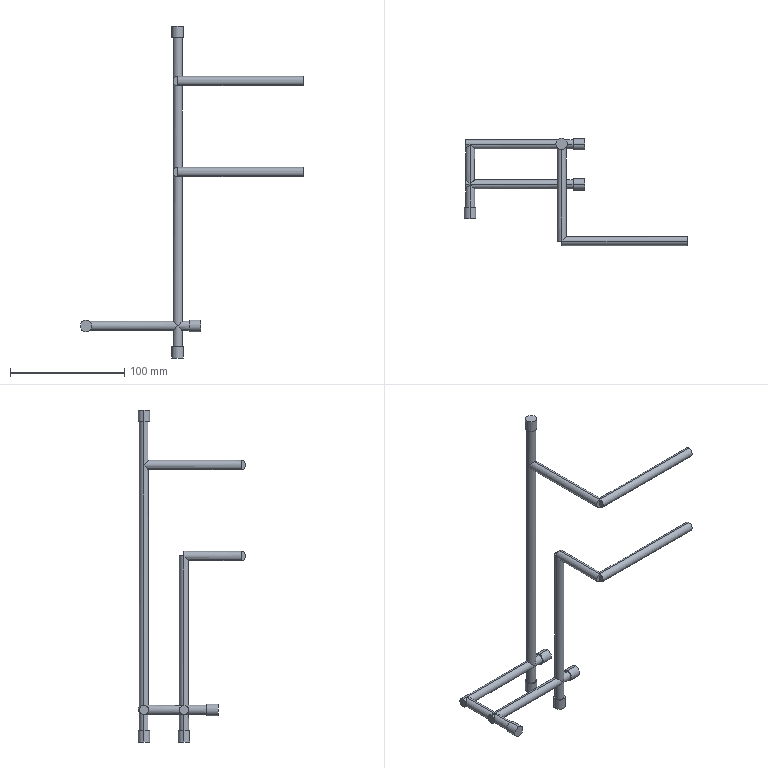Part | STEP file | 1 solid | 68 faces | box 195 x 94 x 290 mm | volume 54387 mm3 | cylinder 46 | plane 22 | commonest cylinder face diameters 8 x34 10 x12